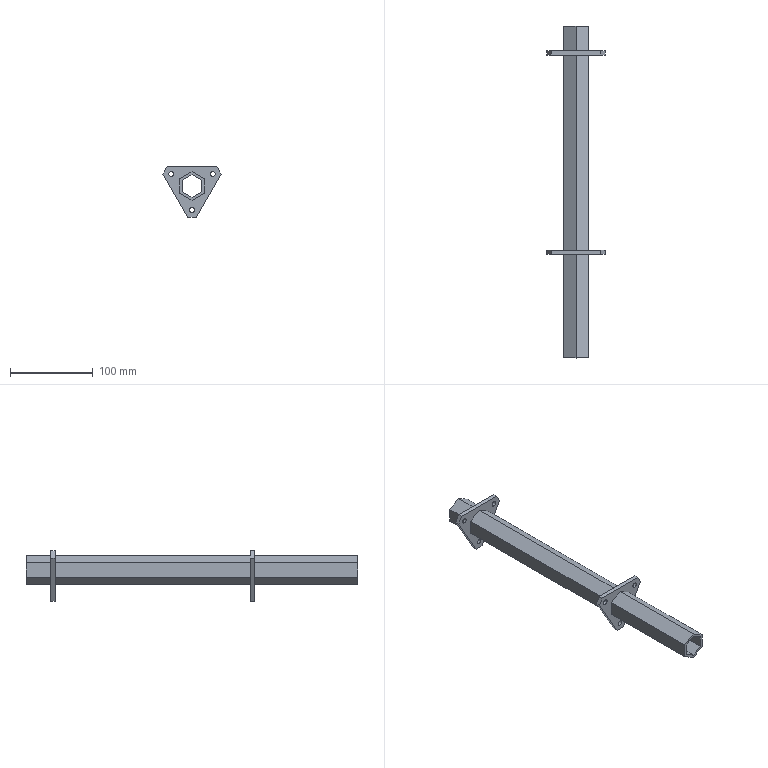Part | SolidWorks | features ICE 5, Extrusion 1, LPattern 1 | 1 solid | 54 faces | box 70 x 400 x 60.622 mm | volume 130008 mm3 | plane 42 | cylinder 12 | commonest cylinder face diameters 6 x12